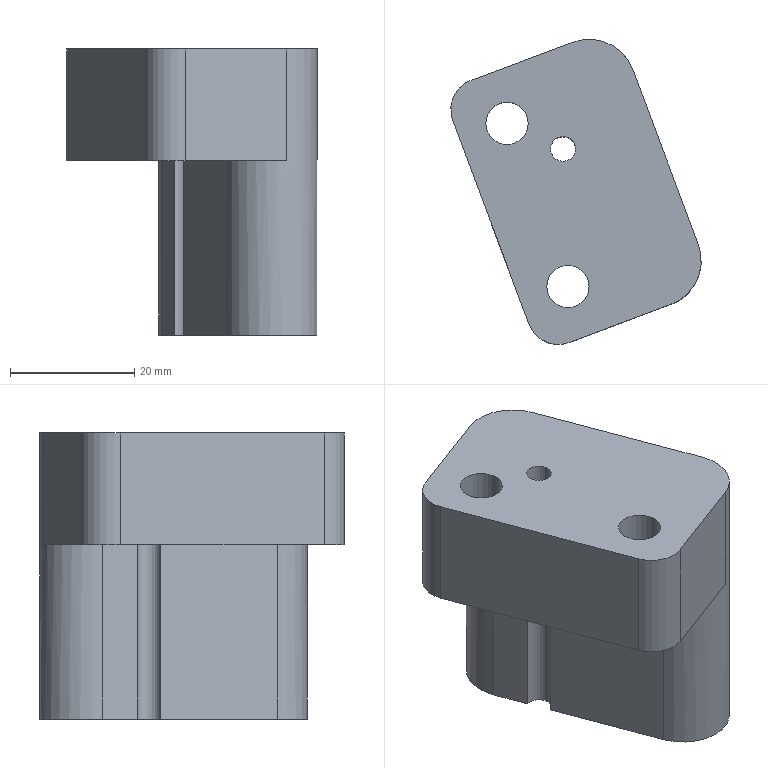Part | NX | features solid 2 | 1 solid | 24 faces | box 40.273 x 49.07 x 46 mm | volume 37890 mm3 | plane 11 | cylinder 11 | cone 2 | commonest cylinder face diameters 5.199 x2 6.8 x2 10 x2 11 x2 15 x2 4.001 x1
STEP:
#1=CARTESIAN_POINT('',(340.887,-34.527,53.002));
#2=VERTEX_POINT('',#1);
#3=CARTESIAN_POINT('',(336.736,-38.135,53.002));
#4=DIRECTION('',(-0.000000102,-0.000000038,-1.));
#5=DIRECTION('',(0.7547,0.6561,-0.000000102));
#6=AXIS2_PLACEMENT_3D('',#3,#4,#5);
#7=CIRCLE('',#6,5.5);
#8=EDGE_CURVE('',#2,#2,#7,.T.);
#9=ORIENTED_EDGE('',*,*,#8,.F.);
#10=EDGE_LOOP('',(#9));
#11=FACE_BOUND('',#10,.T.);
#12=CARTESIAN_POINT('',(342.943,-34.747,53.002));
#13=VERTEX_POINT('',#12);
#14=CARTESIAN_POINT('',(345.044,-40.367,53.002));
#15=VERTEX_POINT('',#14);
#16=CARTESIAN_POINT('',(344.256,-38.26,53.002));
#17=DIRECTION('',(0.3502,-0.9367,0.));
#18=VECTOR('',#17,1000.);
#19=LINE('',#16,#18);
#20=EDGE_CURVE('',#13,#15,#19,.T.);
#21=ORIENTED_EDGE('',*,*,#20,.T.);
#22=CARTESIAN_POINT('',(346.445,-44.114,53.002));
#23=VERTEX_POINT('',#22);
#24=CARTESIAN_POINT('',(345.744,-42.241,53.002));
#25=DIRECTION('',(0.000000102,0.000000038,1.));
#26=DIRECTION('',(-1.,0.,0.000000102));
#27=AXIS2_PLACEMENT_3D('',#24,#25,#26);
#28=CIRCLE('',#27,2.001);
#29=EDGE_CURVE('',#15,#23,#28,.T.);
#30=ORIENTED_EDGE('',*,*,#29,.T.);
#31=CARTESIAN_POINT('',(353.449,-62.847,53.002));
#32=VERTEX_POINT('',#31);
#33=CARTESIAN_POINT('',(344.256,-38.26,53.002));
#34=DIRECTION('',(0.3502,-0.9367,0.));
#35=VECTOR('',#34,1000.);
#36=LINE('',#33,#35);
#37=EDGE_CURVE('',#23,#32,#36,.T.);
#38=ORIENTED_EDGE('',*,*,#37,.T.);
#39=CARTESIAN_POINT('',(363.101,-67.246,53.002));
#40=VERTEX_POINT('',#39);
#41=CARTESIAN_POINT('',(360.474,-60.221,53.002));
#42=DIRECTION('',(0.,0.,-1.));
#43=DIRECTION('',(-1.,0.,0.));
#44=AXIS2_PLACEMENT_3D('',#41,#42,#43);
#45=CIRCLE('',#44,7.5);
#46=EDGE_CURVE('',#40,#32,#45,.T.);
#47=ORIENTED_EDGE('',*,*,#46,.F.);
#48=CARTESIAN_POINT('',(346.709,-73.375,53.002));
#49=VERTEX_POINT('',#48);
#50=CARTESIAN_POINT('',(344.367,-74.25,53.002));
#51=DIRECTION('',(0.9367,0.3502,-0.000000109));
#52=VECTOR('',#51,1000.);
#53=LINE('',#50,#52);
#54=EDGE_CURVE('',#49,#40,#53,.T.);
#55=ORIENTED_EDGE('',*,*,#54,.F.);
#56=CARTESIAN_POINT('',(340.274,-70.442,53.002));
#57=VERTEX_POINT('',#56);
#58=CARTESIAN_POINT('',(344.958,-68.691,53.002));
#59=DIRECTION('',(-0.000000102,-0.000000038,-1.));
#60=DIRECTION('',(-1.,0.,0.000000102));
#61=AXIS2_PLACEMENT_3D('',#58,#59,#60);
#62=CIRCLE('',#61,5.);
#63=EDGE_CURVE('',#49,#57,#62,.T.);
#64=ORIENTED_EDGE('',*,*,#63,.T.);
#65=CARTESIAN_POINT('',(328.017,-37.659,53.002));
#66=VERTEX_POINT('',#65);
#67=CARTESIAN_POINT('',(362.919,-131.008,53.002));
#68=DIRECTION('',(-0.3502,0.9367,0.));
#69=VECTOR('',#68,1000.);
#70=LINE('',#67,#69);
#71=EDGE_CURVE('',#57,#66,#70,.T.);
#72=ORIENTED_EDGE('',*,*,#71,.T.);
#73=CARTESIAN_POINT('',(330.95,-31.224,53.002));
#74=VERTEX_POINT('',#73);
#75=CARTESIAN_POINT('',(332.701,-35.908,53.002));
#76=DIRECTION('',(-0.000000102,-0.000000038,-1.));
#77=DIRECTION('',(-1.,0.,0.000000102));
#78=AXIS2_PLACEMENT_3D('',#75,#76,#77);
#79=CIRCLE('',#78,5.);
#80=EDGE_CURVE('',#66,#74,#79,.T.);
#81=ORIENTED_EDGE('',*,*,#80,.T.);
#82=CARTESIAN_POINT('',(347.341,-25.096,53.002));
#83=VERTEX_POINT('',#82);
#84=CARTESIAN_POINT('',(328.608,-32.1,53.002));
#85=DIRECTION('',(0.9367,0.3502,-0.000000109));
#86=VECTOR('',#85,1000.);
#87=LINE('',#84,#86);
#88=EDGE_CURVE('',#74,#83,#87,.T.);
#89=ORIENTED_EDGE('',*,*,#88,.T.);
#90=CARTESIAN_POINT('',(349.968,-32.121,53.002));
#91=DIRECTION('',(0.,0.,1.));
#92=DIRECTION('',(-1.,0.,0.));
#93=AXIS2_PLACEMENT_3D('',#90,#91,#92);
#94=CIRCLE('',#93,7.5);
#95=EDGE_CURVE('',#83,#13,#94,.T.);
#96=ORIENTED_EDGE('',*,*,#95,.T.);
#97=EDGE_LOOP('',(#21,#30,#38,#47,#55,#64,#72,#81,#89,#96));
#98=FACE_BOUND('',#97,.T.);
#99=CARTESIAN_POINT('',(352.042,-64.362,53.002));
#100=VERTEX_POINT('',#99);
#101=CARTESIAN_POINT('',(346.542,-64.362,53.002));
#102=DIRECTION('',(0.000000102,0.000000038,1.));
#103=DIRECTION('',(1.,0.,-0.000000102));
#104=AXIS2_PLACEMENT_3D('',#101,#102,#103);
#105=CIRCLE('',#104,5.5);
#106=EDGE_CURVE('',#100,#100,#105,.T.);
#107=ORIENTED_EDGE('',*,*,#106,.T.);
#108=EDGE_LOOP('',(#107));
#109=FACE_BOUND('',#108,.T.);
#110=CARTESIAN_POINT('',(365.26,-130.133,53.002));
#111=DIRECTION('',(-0.000000102,-0.000000038,-1.));
#112=DIRECTION('',(1.,0.,-0.000000102));
#113=AXIS2_PLACEMENT_3D('',#110,#111,#112);
#114=PLANE('',#113);
#115=ADVANCED_FACE('',(#11,#98,#109),#114,.T.);
#116=CARTESIAN_POINT('',(340.136,-38.135,71.002));
#117=VERTEX_POINT('',#116);
#118=CARTESIAN_POINT('',(336.736,-38.135,71.002));
#119=DIRECTION('',(0.000000102,0.000000038,1.));
#120=DIRECTION('',(1.,0.,-0.000000102));
#121=AXIS2_PLACEMENT_3D('',#118,#119,#120);
#122=CIRCLE('',#121,3.4);
#123=EDGE_CURVE('',#117,#117,#122,.T.);
#124=ORIENTED_EDGE('',*,*,#123,.F.);
#125=EDGE_LOOP('',(#124));
#126=FACE_BOUND('',#125,.T.);
#127=CARTESIAN_POINT('',(330.95,-31.224,71.002));
#128=VERTEX_POINT('',#127);
#129=CARTESIAN_POINT('',(347.341,-25.096,71.002));
#130=VERTEX_POINT('',#129);
#131=CARTESIAN_POINT('',(328.608,-32.1,71.002));
#132=DIRECTION('',(0.9367,0.3502,-0.000000109));
#133=VECTOR('',#132,1000.);
#134=LINE('',#131,#133);
#135=EDGE_CURVE('',#128,#130,#134,.T.);
#136=ORIENTED_EDGE('',*,*,#135,.F.);
#137=CARTESIAN_POINT('',(328.017,-37.659,71.002));
#138=VERTEX_POINT('',#137);
#139=CARTESIAN_POINT('',(332.701,-35.908,71.002));
#140=DIRECTION('',(0.000000102,0.000000038,1.));
#141=DIRECTION('',(1.,0.,-0.000000102));
#142=AXIS2_PLACEMENT_3D('',#139,#140,#141);
#143=CIRCLE('',#142,5.);
#144=EDGE_CURVE('',#128,#138,#143,.T.);
#145=ORIENTED_EDGE('',*,*,#144,.T.);
#146=CARTESIAN_POINT('',(340.274,-70.442,71.002));
#147=VERTEX_POINT('',#146);
#148=CARTESIAN_POINT('',(362.919,-131.008,71.002));
#149=DIRECTION('',(0.3502,-0.9367,0.));
#150=VECTOR('',#149,1000.);
#151=LINE('',#148,#150);
#152=EDGE_CURVE('',#138,#147,#151,.T.);
#153=ORIENTED_EDGE('',*,*,#152,.T.);
#154=CARTESIAN_POINT('',(346.709,-73.375,71.002));
#155=VERTEX_POINT('',#154);
#156=CARTESIAN_POINT('',(344.958,-68.691,71.002));
#157=DIRECTION('',(0.000000102,0.000000038,1.));
#158=DIRECTION('',(1.,0.,-0.000000102));
#159=AXIS2_PLACEMENT_3D('',#156,#157,#158);
#160=CIRCLE('',#159,5.);
#161=EDGE_CURVE('',#147,#155,#160,.T.);
#162=ORIENTED_EDGE('',*,*,#161,.T.);
#163=CARTESIAN_POINT('',(363.101,-67.246,71.002));
#164=VERTEX_POINT('',#163);
#165=CARTESIAN_POINT('',(344.367,-74.25,71.002));
#166=DIRECTION('',(0.9367,0.3502,-0.000000109));
#167=VECTOR('',#166,1000.);
#168=LINE('',#165,#167);
#169=EDGE_CURVE('',#155,#164,#168,.T.);
#170=ORIENTED_EDGE('',*,*,#169,.T.);
#171=CARTESIAN_POINT('',(367.499,-57.594,71.002));
#172=VERTEX_POINT('',#171);
#173=CARTESIAN_POINT('',(360.474,-60.221,71.002));
#174=DIRECTION('',(0.,0.,-1.));
#175=DIRECTION('',(1.,0.,0.));
#176=AXIS2_PLACEMENT_3D('',#173,#174,#175);
#177=CIRCLE('',#176,7.5);
#178=EDGE_CURVE('',#172,#164,#177,.T.);
#179=ORIENTED_EDGE('',*,*,#178,.F.);
#180=CARTESIAN_POINT('',(356.993,-29.494,71.002));
#181=VERTEX_POINT('',#180);
#182=CARTESIAN_POINT('',(358.306,-33.007,71.002));
#183=DIRECTION('',(0.3502,-0.9367,0.));
#184=VECTOR('',#183,1000.);
#185=LINE('',#182,#184);
#186=EDGE_CURVE('',#181,#172,#185,.T.);
#187=ORIENTED_EDGE('',*,*,#186,.F.);
#188=CARTESIAN_POINT('',(349.968,-32.121,71.002));
#189=DIRECTION('',(0.,0.,-1.));
#190=DIRECTION('',(1.,0.,0.));
#191=AXIS2_PLACEMENT_3D('',#188,#189,#190);
#192=CIRCLE('',#191,7.5);
#193=EDGE_CURVE('',#130,#181,#192,.T.);
#194=ORIENTED_EDGE('',*,*,#193,.F.);
#195=EDGE_LOOP('',(#136,#145,#153,#162,#170,#179,#187,#194));
#196=FACE_BOUND('',#195,.T.);
#197=CARTESIAN_POINT('',(347.745,-42.241,71.002));
#198=VERTEX_POINT('',#197);
#199=CARTESIAN_POINT('',(345.744,-42.241,71.002));
#200=DIRECTION('',(0.000000102,0.000000038,1.));
#201=DIRECTION('',(1.,0.,-0.000000102));
#202=AXIS2_PLACEMENT_3D('',#199,#200,#201);
#203=CIRCLE('',#202,2.001);
#204=EDGE_CURVE('',#198,#198,#203,.T.);
#205=ORIENTED_EDGE('',*,*,#204,.F.);
#206=EDGE_LOOP('',(#205));
#207=FACE_BOUND('',#206,.T.);
#208=CARTESIAN_POINT('',(349.942,-64.362,71.002));
#209=VERTEX_POINT('',#208);
#210=CARTESIAN_POINT('',(346.542,-64.362,71.002));
#211=DIRECTION('',(-0.000000102,-0.000000038,-1.));
#212=DIRECTION('',(1.,0.,-0.000000102));
#213=AXIS2_PLACEMENT_3D('',#210,#211,#212);
#214=CIRCLE('',#213,3.4);
#215=EDGE_CURVE('',#209,#209,#214,.T.);
#216=ORIENTED_EDGE('',*,*,#215,.T.);
#217=EDGE_LOOP('',(#216));
#218=FACE_BOUND('',#217,.T.);
#219=CARTESIAN_POINT('',(365.26,-130.133,71.002));
#220=DIRECTION('',(0.000000102,0.000000038,1.));
#221=DIRECTION('',(-1.,0.,0.000000102));
#222=AXIS2_PLACEMENT_3D('',#219,#220,#221);
#223=PLANE('',#222);
#224=ADVANCED_FACE('',(#126,#196,#207,#218),#223,.T.);
#225=CARTESIAN_POINT('',(346.445,-44.114,25.002));
#226=VERTEX_POINT('',#225);
#227=CARTESIAN_POINT('',(346.445,-44.114,15.002));
#228=DIRECTION('',(0.000000103,0.000000037,1.));
#229=VECTOR('',#228,1000.);
#230=LINE('',#227,#229);
#231=EDGE_CURVE('',#226,#23,#230,.T.);
#232=ORIENTED_EDGE('',*,*,#231,.F.);
#233=CARTESIAN_POINT('',(353.449,-62.847,25.002));
#234=VERTEX_POINT('',#233);
#235=CARTESIAN_POINT('',(344.256,-38.26,25.002));
#236=DIRECTION('',(0.3502,-0.9367,-0.000000001));
#237=VECTOR('',#236,1000.);
#238=LINE('',#235,#237);
#239=EDGE_CURVE('',#226,#234,#238,.T.);
#240=ORIENTED_EDGE('',*,*,#239,.T.);
#241=CARTESIAN_POINT('',(353.449,-62.847,65.002));
#242=DIRECTION('',(-0.000000103,-0.000000037,-1.));
#243=VECTOR('',#242,1000.);
#244=LINE('',#241,#243);
#245=EDGE_CURVE('',#32,#234,#244,.T.);
#246=ORIENTED_EDGE('',*,*,#245,.F.);
#247=ORIENTED_EDGE('',*,*,#37,.F.);
#248=EDGE_LOOP('',(#232,#240,#246,#247));
#249=FACE_BOUND('',#248,.T.);
#250=CARTESIAN_POINT('',(344.256,-38.26,65.002));
#251=DIRECTION('',(0.9367,0.3502,-0.000000109));
#252=DIRECTION('',(0.3502,-0.9367,0.));
#253=AXIS2_PLACEMENT_3D('',#250,#251,#252);
#254=PLANE('',#253);
#255=ADVANCED_FACE('',(#249),#254,.F.);
#256=CARTESIAN_POINT('',(345.044,-40.367,25.002));
#257=VERTEX_POINT('',#256);
#258=CARTESIAN_POINT('',(345.044,-40.367,15.002));
#259=DIRECTION('',(-0.000000103,-0.000000037,-1.));
#260=VECTOR('',#259,1000.);
#261=LINE('',#258,#260);
#262=EDGE_CURVE('',#15,#257,#261,.T.);
#263=ORIENTED_EDGE('',*,*,#262,.F.);
#264=ORIENTED_EDGE('',*,*,#20,.F.);
#265=CARTESIAN_POINT('',(342.943,-34.747,25.002));
#266=VERTEX_POINT('',#265);
#267=CARTESIAN_POINT('',(342.943,-34.747,65.002));
#268=DIRECTION('',(-0.000000103,-0.000000037,-1.));
#269=VECTOR('',#268,1000.);
#270=LINE('',#267,#269);
#271=EDGE_CURVE('',#13,#266,#270,.T.);
#272=ORIENTED_EDGE('',*,*,#271,.T.);
#273=CARTESIAN_POINT('',(344.256,-38.26,25.002));
#274=DIRECTION('',(0.3502,-0.9367,-0.000000001));
#275=VECTOR('',#274,1000.);
#276=LINE('',#273,#275);
#277=EDGE_CURVE('',#266,#257,#276,.T.);
#278=ORIENTED_EDGE('',*,*,#277,.T.);
#279=EDGE_LOOP('',(#263,#264,#272,#278));
#280=FACE_BOUND('',#279,.T.);
#281=CARTESIAN_POINT('',(344.256,-38.26,65.002));
#282=DIRECTION('',(0.9367,0.3502,-0.000000109));
#283=DIRECTION('',(0.3502,-0.9367,0.));
#284=AXIS2_PLACEMENT_3D('',#281,#282,#283);
#285=PLANE('',#284);
#286=ADVANCED_FACE('',(#280),#285,.F.);
#287=CARTESIAN_POINT('',(363.074,-60.221,25.002));
#288=VERTEX_POINT('',#287);
#289=CARTESIAN_POINT('',(360.474,-60.221,25.002));
#290=DIRECTION('',(0.000000103,0.000000037,1.));
#291=DIRECTION('',(1.,0.,-0.000000103));
#292=AXIS2_PLACEMENT_3D('',#289,#290,#291);
#293=CIRCLE('',#292,2.599);
#294=EDGE_CURVE('',#288,#288,#293,.T.);
#295=ORIENTED_EDGE('',*,*,#294,.T.);
#296=EDGE_LOOP('',(#295));
#297=FACE_BOUND('',#296,.T.);
#298=CARTESIAN_POINT('',(352.568,-32.121,25.002));
#299=VERTEX_POINT('',#298);
#300=CARTESIAN_POINT('',(349.968,-32.121,25.002));
#301=DIRECTION('',(0.000000103,0.000000037,1.));
#302=DIRECTION('',(1.,0.,-0.000000103));
#303=AXIS2_PLACEMENT_3D('',#300,#301,#302);
#304=CIRCLE('',#303,2.599);
#305=EDGE_CURVE('',#299,#299,#304,.T.);
#306=ORIENTED_EDGE('',*,*,#305,.T.);
#307=EDGE_LOOP('',(#306));
#308=FACE_BOUND('',#307,.T.);
#309=CARTESIAN_POINT('',(345.744,-42.241,25.002));
#310=DIRECTION('',(-0.000000103,-0.000000037,-1.));
#311=DIRECTION('',(1.,0.,-0.000000103));
#312=AXIS2_PLACEMENT_3D('',#309,#310,#311);
#313=CIRCLE('',#312,2.001);
#314=EDGE_CURVE('',#257,#226,#313,.T.);
#315=ORIENTED_EDGE('',*,*,#314,.F.);
#316=ORIENTED_EDGE('',*,*,#277,.F.);
#317=CARTESIAN_POINT('',(356.993,-29.494,25.002));
#318=VERTEX_POINT('',#317);
#319=CARTESIAN_POINT('',(349.968,-32.121,25.002));
#320=DIRECTION('',(-0.000000103,-0.000000037,-1.));
#321=DIRECTION('',(1.,0.,-0.000000103));
#322=AXIS2_PLACEMENT_3D('',#319,#320,#321);
#323=CIRCLE('',#322,7.5);
#324=EDGE_CURVE('',#266,#318,#323,.T.);
#325=ORIENTED_EDGE('',*,*,#324,.T.);
#326=CARTESIAN_POINT('',(367.499,-57.594,25.002));
#327=VERTEX_POINT('',#326);
#328=CARTESIAN_POINT('',(358.306,-33.007,25.002));
#329=DIRECTION('',(0.3502,-0.9367,-0.000000001));
#330=VECTOR('',#329,1000.);
#331=LINE('',#328,#330);
#332=EDGE_CURVE('',#318,#327,#331,.T.);
#333=ORIENTED_EDGE('',*,*,#332,.T.);
#334=CARTESIAN_POINT('',(360.474,-60.221,25.002));
#335=DIRECTION('',(-0.000000103,-0.000000037,-1.));
#336=DIRECTION('',(1.,0.,-0.000000103));
#337=AXIS2_PLACEMENT_3D('',#334,#335,#336);
#338=CIRCLE('',#337,7.5);
#339=EDGE_CURVE('',#327,#234,#338,.T.);
#340=ORIENTED_EDGE('',*,*,#339,.T.);
#341=ORIENTED_EDGE('',*,*,#239,.F.);
#342=EDGE_LOOP('',(#315,#316,#325,#333,#340,#341));
#343=FACE_BOUND('',#342,.T.);
#344=CARTESIAN_POINT('',(351.281,-35.633,25.002));
#345=DIRECTION('',(0.000000103,0.000000037,1.));
#346=DIRECTION('',(-0.04361,0.999,-0.000000033));
#347=AXIS2_PLACEMENT_3D('',#344,#345,#346);
#348=PLANE('',#347);
#349=ADVANCED_FACE('',(#297,#308,#343),#348,.F.);
#350=ORIENTED_EDGE('',*,*,#95,.F.);
#351=CARTESIAN_POINT('',(347.341,-25.096,65.002));
#352=DIRECTION('',(0.000000103,0.000000037,1.));
#353=VECTOR('',#352,1000.);
#354=LINE('',#351,#353);
#355=EDGE_CURVE('',#83,#130,#354,.T.);
#356=ORIENTED_EDGE('',*,*,#355,.T.);
#357=ORIENTED_EDGE('',*,*,#193,.T.);
#358=CARTESIAN_POINT('',(356.993,-29.494,65.002));
#359=DIRECTION('',(-0.000000103,-0.000000037,-1.));
#360=VECTOR('',#359,1000.);
#361=LINE('',#358,#360);
#362=EDGE_CURVE('',#181,#318,#361,.T.);
#363=ORIENTED_EDGE('',*,*,#362,.T.);
#364=ORIENTED_EDGE('',*,*,#324,.F.);
#365=ORIENTED_EDGE('',*,*,#271,.F.);
#366=EDGE_LOOP('',(#350,#356,#357,#363,#364,#365));
#367=FACE_BOUND('',#366,.T.);
#368=CARTESIAN_POINT('',(349.968,-32.121,65.002));
#369=DIRECTION('',(-0.000000103,-0.000000037,-1.));
#370=DIRECTION('',(1.,0.,-0.000000103));
#371=AXIS2_PLACEMENT_3D('',#368,#369,#370);
#372=CYLINDRICAL_SURFACE('',#371,7.5);
#373=ADVANCED_FACE('',(#367),#372,.T.);
#374=CARTESIAN_POINT('',(367.499,-57.594,65.002));
#375=DIRECTION('',(-0.000000103,-0.000000037,-1.));
#376=VECTOR('',#375,1000.);
#377=LINE('',#374,#376);
#378=EDGE_CURVE('',#172,#327,#377,.T.);
#379=ORIENTED_EDGE('',*,*,#378,.F.);
#380=ORIENTED_EDGE('',*,*,#178,.T.);
#381=CARTESIAN_POINT('',(363.101,-67.246,65.002));
#382=DIRECTION('',(-0.000000103,-0.000000037,-1.));
#383=VECTOR('',#382,1000.);
#384=LINE('',#381,#383);
#385=EDGE_CURVE('',#164,#40,#384,.T.);
#386=ORIENTED_EDGE('',*,*,#385,.T.);
#387=ORIENTED_EDGE('',*,*,#46,.T.);
#388=ORIENTED_EDGE('',*,*,#245,.T.);
#389=ORIENTED_EDGE('',*,*,#339,.F.);
#390=EDGE_LOOP('',(#379,#380,#386,#387,#388,#389));
#391=FACE_BOUND('',#390,.T.);
#392=CARTESIAN_POINT('',(360.474,-60.221,65.002));
#393=DIRECTION('',(-0.000000103,-0.000000037,-1.));
#394=DIRECTION('',(1.,0.,-0.000000103));
#395=AXIS2_PLACEMENT_3D('',#392,#393,#394);
#396=CYLINDRICAL_SURFACE('',#395,7.5);
#397=ADVANCED_FACE('',(#391),#396,.T.);
#398=ORIENTED_EDGE('',*,*,#362,.F.);
#399=ORIENTED_EDGE('',*,*,#186,.T.);
#400=ORIENTED_EDGE('',*,*,#378,.T.);
#401=ORIENTED_EDGE('',*,*,#332,.F.);
#402=EDGE_LOOP('',(#398,#399,#400,#401));
#403=FACE_BOUND('',#402,.T.);
#404=CARTESIAN_POINT('',(358.306,-33.007,65.002));
#405=DIRECTION('',(0.9367,0.3502,-0.000000109));
#406=DIRECTION('',(0.3502,-0.9367,0.));
#407=AXIS2_PLACEMENT_3D('',#404,#405,#406);
#408=PLANE('',#407);
#409=ADVANCED_FACE('',(#403),#408,.T.);
#410=ORIENTED_EDGE('',*,*,#169,.F.);
#411=CARTESIAN_POINT('',(346.709,-73.375,65.002));
#412=DIRECTION('',(-0.000000103,-0.000000037,-1.));
#413=VECTOR('',#412,1000.);
#414=LINE('',#411,#413);
#415=EDGE_CURVE('',#155,#49,#414,.T.);
#416=ORIENTED_EDGE('',*,*,#415,.T.);
#417=ORIENTED_EDGE('',*,*,#54,.T.);
#418=ORIENTED_EDGE('',*,*,#385,.F.);
#419=EDGE_LOOP('',(#410,#416,#417,#418));
#420=FACE_BOUND('',#419,.T.);
#421=CARTESIAN_POINT('',(344.367,-74.25,65.002));
#422=DIRECTION('',(0.3502,-0.9367,-0.000000001));
#423=DIRECTION('',(-0.9367,-0.3502,0.));
#424=AXIS2_PLACEMENT_3D('',#421,#422,#423);
#425=PLANE('',#424);
#426=ADVANCED_FACE('',(#420),#425,.T.);
#427=ORIENTED_EDGE('',*,*,#88,.F.);
#428=CARTESIAN_POINT('',(330.95,-31.224,65.002));
#429=DIRECTION('',(0.000000103,0.000000037,1.));
#430=VECTOR('',#429,1000.);
#431=LINE('',#428,#430);
#432=EDGE_CURVE('',#74,#128,#431,.T.);
#433=ORIENTED_EDGE('',*,*,#432,.T.);
#434=ORIENTED_EDGE('',*,*,#135,.T.);
#435=ORIENTED_EDGE('',*,*,#355,.F.);
#436=EDGE_LOOP('',(#427,#433,#434,#435));
#437=FACE_BOUND('',#436,.T.);
#438=CARTESIAN_POINT('',(328.608,-32.1,65.002));
#439=DIRECTION('',(-0.3502,0.9367,0.000000001));
#440=DIRECTION('',(0.9367,0.3502,0.));
#441=AXIS2_PLACEMENT_3D('',#438,#439,#440);
#442=PLANE('',#441);
#443=ADVANCED_FACE('',(#437),#442,.T.);
#444=ORIENTED_EDGE('',*,*,#152,.F.);
#445=CARTESIAN_POINT('',(328.017,-37.659,53.002));
#446=DIRECTION('',(-0.000000103,-0.000000037,-1.));
#447=VECTOR('',#446,1000.);
#448=LINE('',#445,#447);
#449=EDGE_CURVE('',#138,#66,#448,.T.);
#450=ORIENTED_EDGE('',*,*,#449,.T.);
#451=ORIENTED_EDGE('',*,*,#71,.F.);
#452=CARTESIAN_POINT('',(340.274,-70.442,53.002));
#453=DIRECTION('',(0.000000103,0.000000037,1.));
#454=VECTOR('',#453,1000.);
#455=LINE('',#452,#454);
#456=EDGE_CURVE('',#57,#147,#455,.T.);
#457=ORIENTED_EDGE('',*,*,#456,.T.);
#458=EDGE_LOOP('',(#444,#450,#451,#457));
#459=FACE_BOUND('',#458,.T.);
#460=CARTESIAN_POINT('',(328.893,-40.,53.002));
#461=DIRECTION('',(-0.9367,-0.3502,0.000000109));
#462=DIRECTION('',(-0.3502,0.9367,0.));
#463=AXIS2_PLACEMENT_3D('',#460,#461,#462);
#464=PLANE('',#463);
#465=ADVANCED_FACE('',(#459),#464,.T.);
#466=ORIENTED_EDGE('',*,*,#80,.F.);
#467=ORIENTED_EDGE('',*,*,#449,.F.);
#468=ORIENTED_EDGE('',*,*,#144,.F.);
#469=ORIENTED_EDGE('',*,*,#432,.F.);
#470=EDGE_LOOP('',(#466,#467,#468,#469));
#471=FACE_BOUND('',#470,.T.);
#472=CARTESIAN_POINT('',(332.701,-35.908,65.002));
#473=DIRECTION('',(0.000000103,0.000000037,1.));
#474=DIRECTION('',(-1.,0.,0.000000103));
#475=AXIS2_PLACEMENT_3D('',#472,#473,#474);
#476=CYLINDRICAL_SURFACE('',#475,5.);
#477=ADVANCED_FACE('',(#471),#476,.T.);
#478=ORIENTED_EDGE('',*,*,#161,.F.);
#479=ORIENTED_EDGE('',*,*,#456,.F.);
#480=ORIENTED_EDGE('',*,*,#63,.F.);
#481=ORIENTED_EDGE('',*,*,#415,.F.);
#482=EDGE_LOOP('',(#478,#479,#480,#481));
#483=FACE_BOUND('',#482,.T.);
#484=CARTESIAN_POINT('',(344.958,-68.691,65.002));
#485=DIRECTION('',(-0.000000103,-0.000000037,-1.));
#486=DIRECTION('',(1.,0.,-0.000000103));
#487=AXIS2_PLACEMENT_3D('',#484,#485,#486);
#488=CYLINDRICAL_SURFACE('',#487,5.);
#489=ADVANCED_FACE('',(#483),#488,.T.);
#490=ORIENTED_EDGE('',*,*,#204,.T.);
#491=EDGE_LOOP('',(#490));
#492=FACE_BOUND('',#491,.T.);
#493=ORIENTED_EDGE('',*,*,#314,.T.);
#494=ORIENTED_EDGE('',*,*,#231,.T.);
#495=ORIENTED_EDGE('',*,*,#29,.F.);
#496=ORIENTED_EDGE('',*,*,#262,.T.);
#497=EDGE_LOOP('',(#493,#494,#495,#496));
#498=FACE_BOUND('',#497,.T.);
#499=CARTESIAN_POINT('',(345.744,-42.241,15.002));
#500=DIRECTION('',(-0.000000103,-0.000000037,-1.));
#501=DIRECTION('',(1.,0.,-0.000000103));
#502=AXIS2_PLACEMENT_3D('',#499,#500,#501);
#503=CYLINDRICAL_SURFACE('',#502,2.001);
#504=ADVANCED_FACE('',(#492,#498),#503,.F.);
#505=CARTESIAN_POINT('',(349.942,-64.362,62.002));
#506=VERTEX_POINT('',#505);
#507=CARTESIAN_POINT('',(346.542,-64.362,62.002));
#508=DIRECTION('',(0.000000102,0.000000038,1.));
#509=DIRECTION('',(1.,0.,-0.000000102));
#510=AXIS2_PLACEMENT_3D('',#507,#508,#509);
#511=CIRCLE('',#510,3.4);
#512=EDGE_CURVE('',#506,#506,#511,.T.);
#513=ORIENTED_EDGE('',*,*,#512,.F.);
#514=EDGE_LOOP('',(#513));
#515=FACE_BOUND('',#514,.T.);
#516=ORIENTED_EDGE('',*,*,#215,.F.);
#517=EDGE_LOOP('',(#516));
#518=FACE_BOUND('',#517,.T.);
#519=CARTESIAN_POINT('',(346.542,-64.362,53.002));
#520=DIRECTION('',(0.000000102,0.000000038,1.));
#521=DIRECTION('',(-1.,0.,0.000000102));
#522=AXIS2_PLACEMENT_3D('',#519,#520,#521);
#523=CYLINDRICAL_SURFACE('',#522,3.4);
#524=ADVANCED_FACE('',(#515,#518),#523,.F.);
#525=ORIENTED_EDGE('',*,*,#512,.T.);
#526=EDGE_LOOP('',(#525));
#527=FACE_BOUND('',#526,.T.);
#528=CARTESIAN_POINT('',(352.042,-64.362,62.002));
#529=VERTEX_POINT('',#528);
#530=CARTESIAN_POINT('',(346.542,-64.362,62.002));
#531=DIRECTION('',(0.000000102,0.000000038,1.));
#532=DIRECTION('',(1.,0.,-0.000000102));
#533=AXIS2_PLACEMENT_3D('',#530,#531,#532);
#534=CIRCLE('',#533,5.5);
#535=EDGE_CURVE('',#529,#529,#534,.T.);
#536=ORIENTED_EDGE('',*,*,#535,.F.);
#537=EDGE_LOOP('',(#536));
#538=FACE_BOUND('',#537,.T.);
#539=CARTESIAN_POINT('',(346.542,-64.362,62.002));
#540=DIRECTION('',(0.000000102,0.000000038,1.));
#541=DIRECTION('',(-1.,0.,0.000000102));
#542=AXIS2_PLACEMENT_3D('',#539,#540,#541);
#543=PLANE('',#542);
#544=ADVANCED_FACE('',(#527,#538),#543,.F.);
#545=ORIENTED_EDGE('',*,*,#535,.T.);
#546=EDGE_LOOP('',(#545));
#547=FACE_BOUND('',#546,.T.);
#548=ORIENTED_EDGE('',*,*,#106,.F.);
#549=EDGE_LOOP('',(#548));
#550=FACE_BOUND('',#549,.T.);
#551=CARTESIAN_POINT('',(346.542,-64.362,53.002));
#552=DIRECTION('',(0.000000102,0.000000038,1.));
#553=DIRECTION('',(-1.,0.,0.000000102));
#554=AXIS2_PLACEMENT_3D('',#551,#552,#553);
#555=CYLINDRICAL_SURFACE('',#554,5.5);
#556=ADVANCED_FACE('',(#547,#550),#555,.F.);
#557=CARTESIAN_POINT('',(340.136,-38.135,62.002));
#558=VERTEX_POINT('',#557);
#559=CARTESIAN_POINT('',(336.736,-38.135,62.002));
#560=DIRECTION('',(-0.000000102,-0.000000038,-1.));
#561=DIRECTION('',(1.,0.,-0.000000102));
#562=AXIS2_PLACEMENT_3D('',#559,#560,#561);
#563=CIRCLE('',#562,3.4);
#564=EDGE_CURVE('',#558,#558,#563,.T.);
#565=ORIENTED_EDGE('',*,*,#564,.T.);
#566=EDGE_LOOP('',(#565));
#567=FACE_BOUND('',#566,.T.);
#568=ORIENTED_EDGE('',*,*,#123,.T.);
#569=EDGE_LOOP('',(#568));
#570=FACE_BOUND('',#569,.T.);
#571=CARTESIAN_POINT('',(336.736,-38.135,53.002));
#572=DIRECTION('',(0.000000102,0.000000038,1.));
#573=DIRECTION('',(-0.7547,-0.6561,0.000000102));
#574=AXIS2_PLACEMENT_3D('',#571,#572,#573);
#575=CYLINDRICAL_SURFACE('',#574,3.4);
#576=ADVANCED_FACE('',(#567,#570),#575,.F.);
#577=ORIENTED_EDGE('',*,*,#564,.F.);
#578=EDGE_LOOP('',(#577));
#579=FACE_BOUND('',#578,.T.);
#580=CARTESIAN_POINT('',(340.887,-34.527,62.002));
#581=VERTEX_POINT('',#580);
#582=CARTESIAN_POINT('',(336.736,-38.135,62.002));
#583=DIRECTION('',(-0.000000102,-0.000000038,-1.));
#584=DIRECTION('',(0.7547,0.6561,-0.000000102));
#585=AXIS2_PLACEMENT_3D('',#582,#583,#584);
#586=CIRCLE('',#585,5.5);
#587=EDGE_CURVE('',#581,#581,#586,.T.);
#588=ORIENTED_EDGE('',*,*,#587,.T.);
#589=EDGE_LOOP('',(#588));
#590=FACE_BOUND('',#589,.T.);
#591=CARTESIAN_POINT('',(336.736,-38.135,62.002));
#592=DIRECTION('',(0.000000102,0.000000038,1.));
#593=DIRECTION('',(-0.7547,-0.6561,0.000000102));
#594=AXIS2_PLACEMENT_3D('',#591,#592,#593);
#595=PLANE('',#594);
#596=ADVANCED_FACE('',(#579,#590),#595,.F.);
#597=ORIENTED_EDGE('',*,*,#587,.F.);
#598=EDGE_LOOP('',(#597));
#599=FACE_BOUND('',#598,.T.);
#600=ORIENTED_EDGE('',*,*,#8,.T.);
#601=EDGE_LOOP('',(#600));
#602=FACE_BOUND('',#601,.T.);
#603=CARTESIAN_POINT('',(336.736,-38.135,53.002));
#604=DIRECTION('',(0.000000102,0.000000038,1.));
#605=DIRECTION('',(-0.7547,-0.6561,0.000000102));
#606=AXIS2_PLACEMENT_3D('',#603,#604,#605);
#607=CYLINDRICAL_SURFACE('',#606,5.5);
#608=ADVANCED_FACE('',(#599,#602),#607,.F.);
#609=CARTESIAN_POINT('',(352.568,-32.121,37.403));
#610=VERTEX_POINT('',#609);
#611=CARTESIAN_POINT('',(349.968,-32.121,37.403));
#612=DIRECTION('',(0.000000103,0.000000037,1.));
#613=DIRECTION('',(1.,0.,-0.000000103));
#614=AXIS2_PLACEMENT_3D('',#611,#612,#613);
#615=CIRCLE('',#614,2.599);
#616=EDGE_CURVE('',#610,#610,#615,.T.);
#617=ORIENTED_EDGE('',*,*,#616,.T.);
#618=EDGE_LOOP('',(#617));
#619=FACE_BOUND('',#618,.T.);
#620=ORIENTED_EDGE('',*,*,#305,.F.);
#621=EDGE_LOOP('',(#620));
#622=FACE_BOUND('',#621,.T.);
#623=CARTESIAN_POINT('',(349.968,-32.121,25.002));
#624=DIRECTION('',(0.000000103,0.000000037,1.));
#625=DIRECTION('',(-1.,0.,0.000000103));
#626=AXIS2_PLACEMENT_3D('',#623,#624,#625);
#627=CYLINDRICAL_SURFACE('',#626,2.599);
#628=ADVANCED_FACE('',(#619,#622),#627,.F.);
#629=CARTESIAN_POINT('',(349.968,-32.121,40.002));
#630=VERTEX_POINT('',#629);
#631=VERTEX_LOOP('',#630);
#632=FACE_BOUND('',#631,.T.);
#633=ORIENTED_EDGE('',*,*,#616,.F.);
#634=EDGE_LOOP('',(#633));
#635=FACE_BOUND('',#634,.T.);
#636=CARTESIAN_POINT('',(349.968,-32.121,37.403));
#637=DIRECTION('',(-0.000000103,-0.000000037,-1.));
#638=DIRECTION('',(1.,0.,-0.000000103));
#639=AXIS2_PLACEMENT_3D('',#636,#637,#638);
#640=CONICAL_SURFACE('',#639,2.599,0.7854);
#641=ADVANCED_FACE('',(#632,#635),#640,.F.);
#642=CARTESIAN_POINT('',(363.074,-60.221,37.403));
#643=VERTEX_POINT('',#642);
#644=CARTESIAN_POINT('',(360.474,-60.221,37.403));
#645=DIRECTION('',(0.000000103,0.000000037,1.));
#646=DIRECTION('',(1.,0.,-0.000000103));
#647=AXIS2_PLACEMENT_3D('',#644,#645,#646);
#648=CIRCLE('',#647,2.599);
#649=EDGE_CURVE('',#643,#643,#648,.T.);
#650=ORIENTED_EDGE('',*,*,#649,.T.);
#651=EDGE_LOOP('',(#650));
#652=FACE_BOUND('',#651,.T.);
#653=ORIENTED_EDGE('',*,*,#294,.F.);
#654=EDGE_LOOP('',(#653));
#655=FACE_BOUND('',#654,.T.);
#656=CARTESIAN_POINT('',(360.474,-60.221,25.002));
#657=DIRECTION('',(0.000000103,0.000000037,1.));
#658=DIRECTION('',(-1.,0.,0.000000103));
#659=AXIS2_PLACEMENT_3D('',#656,#657,#658);
#660=CYLINDRICAL_SURFACE('',#659,2.599);
#661=ADVANCED_FACE('',(#652,#655),#660,.F.);
#662=CARTESIAN_POINT('',(360.474,-60.221,40.002));
#663=VERTEX_POINT('',#662);
#664=VERTEX_LOOP('',#663);
#665=FACE_BOUND('',#664,.T.);
#666=ORIENTED_EDGE('',*,*,#649,.F.);
#667=EDGE_LOOP('',(#666));
#668=FACE_BOUND('',#667,.T.);
#669=CARTESIAN_POINT('',(360.474,-60.221,37.403));
#670=DIRECTION('',(-0.000000103,-0.000000037,-1.));
#671=DIRECTION('',(1.,0.,-0.000000103));
#672=AXIS2_PLACEMENT_3D('',#669,#670,#671);
#673=CONICAL_SURFACE('',#672,2.599,0.7854);
#674=ADVANCED_FACE('',(#665,#668),#673,.F.);
#675=CLOSED_SHELL('',(#115,#224,#255,#286,#349,#373,#397,#409,#426,#443,#465,#477,#489,#504,#524,#544,#556,#576,#596,#608,#628,#641,#661,#674));
#676=MANIFOLD_SOLID_BREP('',#675);
#677=(LENGTH_UNIT()NAMED_UNIT(*)SI_UNIT(.MILLI.,.METRE.));
#678=UNCERTAINTY_MEASURE_WITH_UNIT(LENGTH_MEASURE(0.00001),#677,'','');
#679=(NAMED_UNIT(*)PLANE_ANGLE_UNIT()SI_UNIT($,.RADIAN.));
#680=(NAMED_UNIT(*)SI_UNIT($,.STERADIAN.)SOLID_ANGLE_UNIT());
#681=(GEOMETRIC_REPRESENTATION_CONTEXT(3)GLOBAL_UNCERTAINTY_ASSIGNED_CONTEXT((#678))GLOBAL_UNIT_ASSIGNED_CONTEXT((#677,#679,#680))REPRESENTATION_CONTEXT('',''));
#682=ADVANCED_BREP_SHAPE_REPRESENTATION('',(#676),#681);